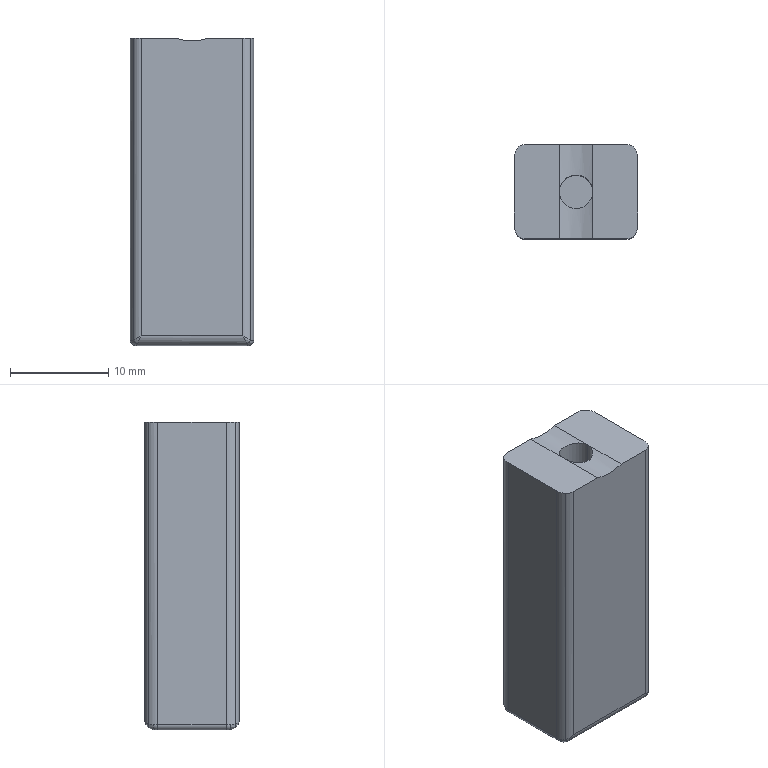Part | SolidWorks | features BaseBody 1 | 1 solid | 37 faces | box 12.534 x 9.6 x 31.25 mm | volume 3446 mm3 | cylinder 17 | plane 8 | spline 8 | torus 4 | commonest cylinder face diameters 2 x6 3 x5 1 x2 3.4 x2 10 x2